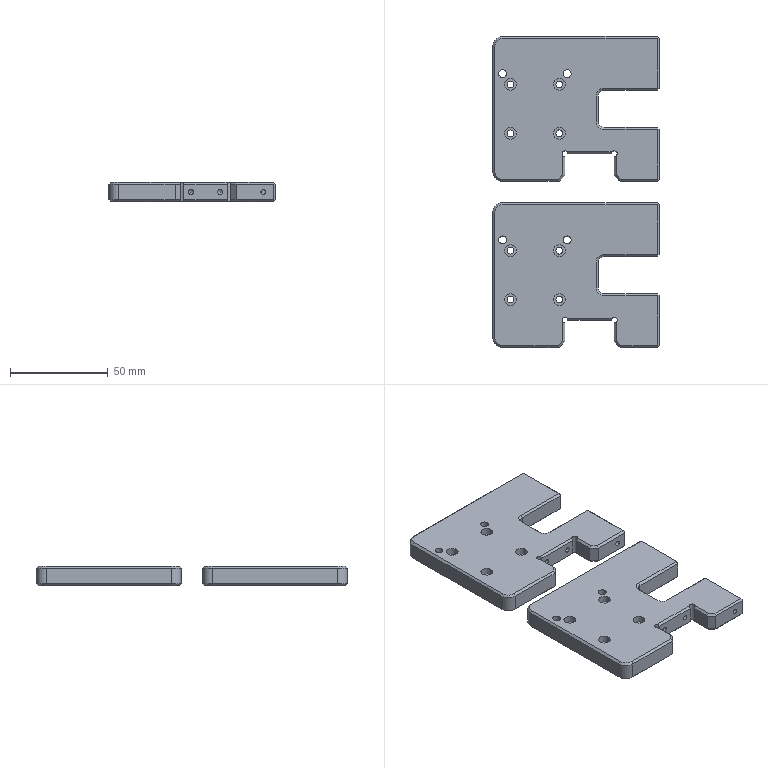Part | 2 solids | 184 faces | box 85 x 159 x 10 mm | volume 101673 mm3 | plane 116 | cylinder 48 | cone 12 | spline 8 | commonest cylinder face diameters 6 x16 2.5 x12 3.5 x8 3 x4 4 x4 10 x4